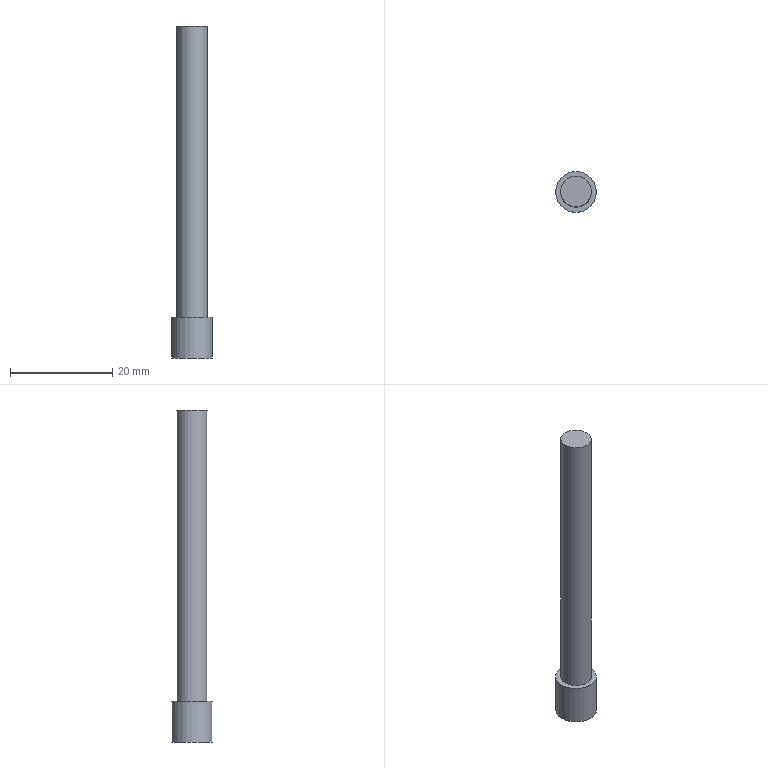Part | NX | features solid 2 | 1 solid | 5 faces | box 8 x 8 x 65 mm | volume 2014 mm3 | plane 3 | cylinder 2 | commonest cylinder face diameters 6 x1 8 x1
STEP:
#1=CARTESIAN_POINT('',(-30.,72.,30.));
#2=VERTEX_POINT('',#1);
#3=CARTESIAN_POINT('',(-27.,72.,30.));
#4=DIRECTION('',(0.,0.,1.));
#5=DIRECTION('',(-1.,0.,0.));
#6=AXIS2_PLACEMENT_3D('',#3,#4,#5);
#7=CIRCLE('',#6,3.);
#8=EDGE_CURVE('',#2,#2,#7,.F.);
#9=ORIENTED_EDGE('',*,*,#8,.T.);
#10=EDGE_LOOP('',(#9));
#11=FACE_BOUND('',#10,.T.);
#12=CARTESIAN_POINT('',(-24.,72.,-27.));
#13=VERTEX_POINT('',#12);
#14=CARTESIAN_POINT('',(-27.,72.,-27.));
#15=DIRECTION('',(0.,0.,1.));
#16=DIRECTION('',(1.,0.,0.));
#17=AXIS2_PLACEMENT_3D('',#14,#15,#16);
#18=CIRCLE('',#17,3.);
#19=EDGE_CURVE('',#13,#13,#18,.F.);
#20=ORIENTED_EDGE('',*,*,#19,.F.);
#21=EDGE_LOOP('',(#20));
#22=FACE_BOUND('',#21,.T.);
#23=CARTESIAN_POINT('',(-27.,72.,25.));
#24=DIRECTION('',(0.,0.,-1.));
#25=DIRECTION('',(-1.,0.,0.));
#26=AXIS2_PLACEMENT_3D('',#23,#24,#25);
#27=CYLINDRICAL_SURFACE('',#26,3.);
#28=ADVANCED_FACE('',(#11,#22),#27,.T.);
#29=ORIENTED_EDGE('',*,*,#8,.F.);
#30=EDGE_LOOP('',(#29));
#31=FACE_BOUND('',#30,.T.);
#32=CARTESIAN_POINT('',(-27.,72.,30.));
#33=DIRECTION('',(0.,0.,1.));
#34=DIRECTION('',(-1.,0.,0.));
#35=AXIS2_PLACEMENT_3D('',#32,#33,#34);
#36=PLANE('',#35);
#37=ADVANCED_FACE('',(#31),#36,.T.);
#38=CARTESIAN_POINT('',(-23.,72.,-27.));
#39=VERTEX_POINT('',#38);
#40=CARTESIAN_POINT('',(-27.,72.,-27.));
#41=DIRECTION('',(0.,0.,1.));
#42=DIRECTION('',(1.,0.,0.));
#43=AXIS2_PLACEMENT_3D('',#40,#41,#42);
#44=CIRCLE('',#43,4.);
#45=EDGE_CURVE('',#39,#39,#44,.T.);
#46=ORIENTED_EDGE('',*,*,#45,.F.);
#47=EDGE_LOOP('',(#46));
#48=FACE_BOUND('',#47,.T.);
#49=CARTESIAN_POINT('',(-23.,72.,-35.));
#50=VERTEX_POINT('',#49);
#51=CARTESIAN_POINT('',(-27.,72.,-35.));
#52=DIRECTION('',(0.,0.,1.));
#53=DIRECTION('',(1.,0.,0.));
#54=AXIS2_PLACEMENT_3D('',#51,#52,#53);
#55=CIRCLE('',#54,4.);
#56=EDGE_CURVE('',#50,#50,#55,.T.);
#57=ORIENTED_EDGE('',*,*,#56,.T.);
#58=EDGE_LOOP('',(#57));
#59=FACE_BOUND('',#58,.T.);
#60=CARTESIAN_POINT('',(-27.,72.,-27.));
#61=DIRECTION('',(0.,0.,-1.));
#62=DIRECTION('',(1.,0.,0.));
#63=AXIS2_PLACEMENT_3D('',#60,#61,#62);
#64=CYLINDRICAL_SURFACE('',#63,4.);
#65=ADVANCED_FACE('',(#48,#59),#64,.T.);
#66=ORIENTED_EDGE('',*,*,#19,.T.);
#67=EDGE_LOOP('',(#66));
#68=FACE_BOUND('',#67,.T.);
#69=ORIENTED_EDGE('',*,*,#45,.T.);
#70=EDGE_LOOP('',(#69));
#71=FACE_BOUND('',#70,.T.);
#72=CARTESIAN_POINT('',(-27.,72.,-27.));
#73=DIRECTION('',(0.,0.,-1.));
#74=DIRECTION('',(1.,0.,0.));
#75=AXIS2_PLACEMENT_3D('',#72,#73,#74);
#76=PLANE('',#75);
#77=ADVANCED_FACE('',(#68,#71),#76,.F.);
#78=ORIENTED_EDGE('',*,*,#56,.F.);
#79=EDGE_LOOP('',(#78));
#80=FACE_BOUND('',#79,.T.);
#81=CARTESIAN_POINT('',(-8.802,-48.336,-35.));
#82=DIRECTION('',(0.,0.,1.));
#83=DIRECTION('',(1.,0.,0.));
#84=AXIS2_PLACEMENT_3D('',#81,#82,#83);
#85=PLANE('',#84);
#86=ADVANCED_FACE('',(#80),#85,.F.);
#87=CLOSED_SHELL('',(#28,#37,#65,#77,#86));
#88=MANIFOLD_SOLID_BREP('',#87);
#89=(LENGTH_UNIT()NAMED_UNIT(*)SI_UNIT(.MILLI.,.METRE.));
#90=UNCERTAINTY_MEASURE_WITH_UNIT(LENGTH_MEASURE(0.00001),#89,'','');
#91=(NAMED_UNIT(*)PLANE_ANGLE_UNIT()SI_UNIT($,.RADIAN.));
#92=(NAMED_UNIT(*)SI_UNIT($,.STERADIAN.)SOLID_ANGLE_UNIT());
#93=(GEOMETRIC_REPRESENTATION_CONTEXT(3)GLOBAL_UNCERTAINTY_ASSIGNED_CONTEXT((#90))GLOBAL_UNIT_ASSIGNED_CONTEXT((#89,#91,#92))REPRESENTATION_CONTEXT('',''));
#94=ADVANCED_BREP_SHAPE_REPRESENTATION('',(#88),#93);